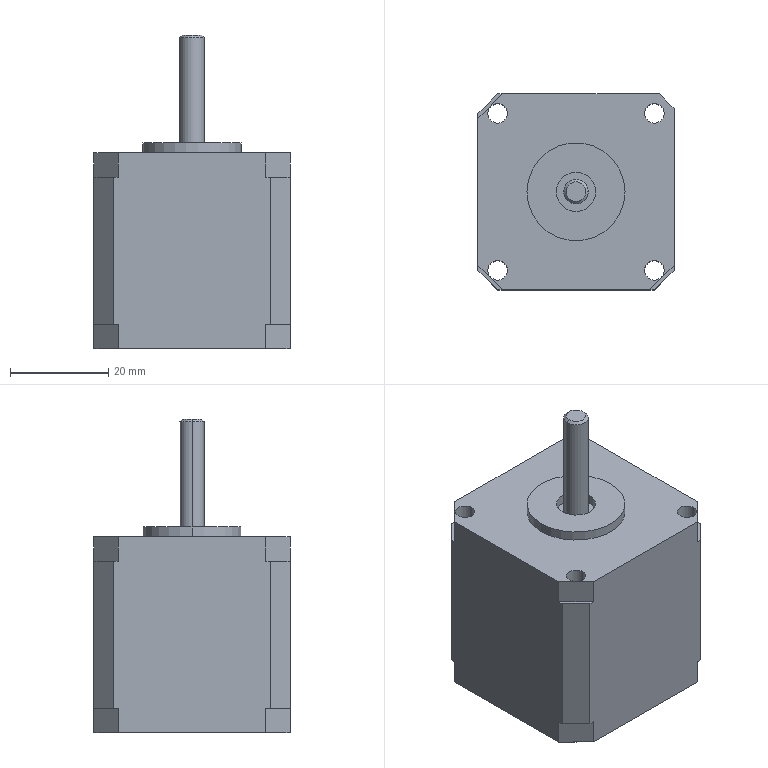Part | SolidWorks | features ICE 5, Chamfer 2, Extrusion 1, MirrorPattern 1 | 1 solid | 45 faces | box 40 x 40 x 64 mm | volume 61607 mm3 | plane 29 | cylinder 14 | cone 2 | commonest cylinder face diameters 4 x8 5 x2 8 x2 20 x2
STEP:
#1=CARTESIAN_POINT('',(-18.,16.,-20.));
#2=VERTEX_POINT('',#1);
#3=CARTESIAN_POINT('',(-14.,16.,-20.));
#4=VERTEX_POINT('',#3);
#5=CARTESIAN_POINT('',(-16.,16.,-20.));
#6=DIRECTION('',(0.,0.,1.));
#7=DIRECTION('',(1.,0.,0.));
#8=AXIS2_PLACEMENT_3D('',#5,#6,#7);
#9=CIRCLE('',#8,2.);
#10=EDGE_CURVE('',#2,#4,#9,.T.);
#11=ORIENTED_EDGE('',*,*,#10,.F.);
#12=CARTESIAN_POINT('',(-18.,16.,20.));
#13=VERTEX_POINT('',#12);
#14=CARTESIAN_POINT('',(-18.,16.,-20.));
#15=DIRECTION('',(0.,0.,1.));
#16=VECTOR('',#15,1000.);
#17=LINE('',#14,#16);
#18=EDGE_CURVE('',#2,#13,#17,.T.);
#19=ORIENTED_EDGE('',*,*,#18,.T.);
#20=CARTESIAN_POINT('',(-14.,16.,20.));
#21=VERTEX_POINT('',#20);
#22=CARTESIAN_POINT('',(-16.,16.,20.));
#23=DIRECTION('',(0.,0.,1.));
#24=DIRECTION('',(1.,0.,0.));
#25=AXIS2_PLACEMENT_3D('',#22,#23,#24);
#26=CIRCLE('',#25,2.);
#27=EDGE_CURVE('',#13,#21,#26,.T.);
#28=ORIENTED_EDGE('',*,*,#27,.T.);
#29=CARTESIAN_POINT('',(-14.,16.,-20.));
#30=DIRECTION('',(0.,0.,1.));
#31=VECTOR('',#30,1000.);
#32=LINE('',#29,#31);
#33=EDGE_CURVE('',#4,#21,#32,.T.);
#34=ORIENTED_EDGE('',*,*,#33,.F.);
#35=EDGE_LOOP('',(#11,#19,#28,#34));
#36=FACE_OUTER_BOUND('',#35,.T.);
#37=CARTESIAN_POINT('',(-16.,16.,-20.));
#38=DIRECTION('',(0.,0.,1.));
#39=DIRECTION('',(1.,0.,0.));
#40=AXIS2_PLACEMENT_3D('',#37,#38,#39);
#41=CYLINDRICAL_SURFACE('',#40,2.);
#42=ADVANCED_FACE('',(#36),#41,.F.);
#43=CARTESIAN_POINT('',(-18.,-16.,-20.));
#44=VERTEX_POINT('',#43);
#45=CARTESIAN_POINT('',(-14.,-16.,-20.));
#46=VERTEX_POINT('',#45);
#47=CARTESIAN_POINT('',(-16.,-16.,-20.));
#48=DIRECTION('',(0.,0.,1.));
#49=DIRECTION('',(1.,0.,0.));
#50=AXIS2_PLACEMENT_3D('',#47,#48,#49);
#51=CIRCLE('',#50,2.);
#52=EDGE_CURVE('',#44,#46,#51,.T.);
#53=ORIENTED_EDGE('',*,*,#52,.F.);
#54=CARTESIAN_POINT('',(-18.,-16.,20.));
#55=VERTEX_POINT('',#54);
#56=CARTESIAN_POINT('',(-18.,-16.,-20.));
#57=DIRECTION('',(0.,0.,1.));
#58=VECTOR('',#57,1000.);
#59=LINE('',#56,#58);
#60=EDGE_CURVE('',#44,#55,#59,.T.);
#61=ORIENTED_EDGE('',*,*,#60,.T.);
#62=CARTESIAN_POINT('',(-14.,-16.,20.));
#63=VERTEX_POINT('',#62);
#64=CARTESIAN_POINT('',(-16.,-16.,20.));
#65=DIRECTION('',(0.,0.,1.));
#66=DIRECTION('',(1.,0.,0.));
#67=AXIS2_PLACEMENT_3D('',#64,#65,#66);
#68=CIRCLE('',#67,2.);
#69=EDGE_CURVE('',#55,#63,#68,.T.);
#70=ORIENTED_EDGE('',*,*,#69,.T.);
#71=CARTESIAN_POINT('',(-14.,-16.,-20.));
#72=DIRECTION('',(0.,0.,1.));
#73=VECTOR('',#72,1000.);
#74=LINE('',#71,#73);
#75=EDGE_CURVE('',#46,#63,#74,.T.);
#76=ORIENTED_EDGE('',*,*,#75,.F.);
#77=EDGE_LOOP('',(#53,#61,#70,#76));
#78=FACE_OUTER_BOUND('',#77,.T.);
#79=CARTESIAN_POINT('',(-16.,-16.,-20.));
#80=DIRECTION('',(0.,0.,1.));
#81=DIRECTION('',(1.,0.,0.));
#82=AXIS2_PLACEMENT_3D('',#79,#80,#81);
#83=CYLINDRICAL_SURFACE('',#82,2.);
#84=ADVANCED_FACE('',(#78),#83,.F.);
#85=CARTESIAN_POINT('',(14.,-16.,-20.));
#86=VERTEX_POINT('',#85);
#87=CARTESIAN_POINT('',(18.,-16.,-20.));
#88=VERTEX_POINT('',#87);
#89=CARTESIAN_POINT('',(16.,-16.,-20.));
#90=DIRECTION('',(0.,0.,1.));
#91=DIRECTION('',(1.,0.,0.));
#92=AXIS2_PLACEMENT_3D('',#89,#90,#91);
#93=CIRCLE('',#92,2.);
#94=EDGE_CURVE('',#86,#88,#93,.T.);
#95=ORIENTED_EDGE('',*,*,#94,.F.);
#96=CARTESIAN_POINT('',(14.,-16.,20.));
#97=VERTEX_POINT('',#96);
#98=CARTESIAN_POINT('',(14.,-16.,-20.));
#99=DIRECTION('',(0.,0.,1.));
#100=VECTOR('',#99,1000.);
#101=LINE('',#98,#100);
#102=EDGE_CURVE('',#86,#97,#101,.T.);
#103=ORIENTED_EDGE('',*,*,#102,.T.);
#104=CARTESIAN_POINT('',(18.,-16.,20.));
#105=VERTEX_POINT('',#104);
#106=CARTESIAN_POINT('',(16.,-16.,20.));
#107=DIRECTION('',(0.,0.,1.));
#108=DIRECTION('',(1.,0.,0.));
#109=AXIS2_PLACEMENT_3D('',#106,#107,#108);
#110=CIRCLE('',#109,2.);
#111=EDGE_CURVE('',#97,#105,#110,.T.);
#112=ORIENTED_EDGE('',*,*,#111,.T.);
#113=CARTESIAN_POINT('',(18.,-16.,-20.));
#114=DIRECTION('',(0.,0.,1.));
#115=VECTOR('',#114,1000.);
#116=LINE('',#113,#115);
#117=EDGE_CURVE('',#88,#105,#116,.T.);
#118=ORIENTED_EDGE('',*,*,#117,.F.);
#119=EDGE_LOOP('',(#95,#103,#112,#118));
#120=FACE_OUTER_BOUND('',#119,.T.);
#121=CARTESIAN_POINT('',(16.,-16.,-20.));
#122=DIRECTION('',(0.,0.,1.));
#123=DIRECTION('',(1.,0.,0.));
#124=AXIS2_PLACEMENT_3D('',#121,#122,#123);
#125=CYLINDRICAL_SURFACE('',#124,2.);
#126=ADVANCED_FACE('',(#120),#125,.F.);
#127=CARTESIAN_POINT('',(14.,16.,-20.));
#128=VERTEX_POINT('',#127);
#129=CARTESIAN_POINT('',(18.,16.,-20.));
#130=VERTEX_POINT('',#129);
#131=CARTESIAN_POINT('',(16.,16.,-20.));
#132=DIRECTION('',(0.,0.,1.));
#133=DIRECTION('',(1.,0.,0.));
#134=AXIS2_PLACEMENT_3D('',#131,#132,#133);
#135=CIRCLE('',#134,2.);
#136=EDGE_CURVE('',#128,#130,#135,.T.);
#137=ORIENTED_EDGE('',*,*,#136,.F.);
#138=CARTESIAN_POINT('',(14.,16.,20.));
#139=VERTEX_POINT('',#138);
#140=CARTESIAN_POINT('',(14.,16.,-20.));
#141=DIRECTION('',(0.,0.,1.));
#142=VECTOR('',#141,1000.);
#143=LINE('',#140,#142);
#144=EDGE_CURVE('',#128,#139,#143,.T.);
#145=ORIENTED_EDGE('',*,*,#144,.T.);
#146=CARTESIAN_POINT('',(18.,16.,20.));
#147=VERTEX_POINT('',#146);
#148=CARTESIAN_POINT('',(16.,16.,20.));
#149=DIRECTION('',(0.,0.,1.));
#150=DIRECTION('',(1.,0.,0.));
#151=AXIS2_PLACEMENT_3D('',#148,#149,#150);
#152=CIRCLE('',#151,2.);
#153=EDGE_CURVE('',#139,#147,#152,.T.);
#154=ORIENTED_EDGE('',*,*,#153,.T.);
#155=CARTESIAN_POINT('',(18.,16.,-20.));
#156=DIRECTION('',(0.,0.,1.));
#157=VECTOR('',#156,1000.);
#158=LINE('',#155,#157);
#159=EDGE_CURVE('',#130,#147,#158,.T.);
#160=ORIENTED_EDGE('',*,*,#159,.F.);
#161=EDGE_LOOP('',(#137,#145,#154,#160));
#162=FACE_OUTER_BOUND('',#161,.T.);
#163=CARTESIAN_POINT('',(16.,16.,-20.));
#164=DIRECTION('',(0.,0.,1.));
#165=DIRECTION('',(1.,0.,0.));
#166=AXIS2_PLACEMENT_3D('',#163,#164,#165);
#167=CYLINDRICAL_SURFACE('',#166,2.);
#168=ADVANCED_FACE('',(#162),#167,.F.);
#169=CARTESIAN_POINT('',(2.,0.,44.));
#170=VERTEX_POINT('',#169);
#171=CARTESIAN_POINT('',(-2.,0.,44.));
#172=VERTEX_POINT('',#171);
#173=CARTESIAN_POINT('',(0.,0.,44.));
#174=DIRECTION('',(0.,0.,1.));
#175=DIRECTION('',(1.,0.,0.));
#176=AXIS2_PLACEMENT_3D('',#173,#174,#175);
#177=CIRCLE('',#176,2.);
#178=EDGE_CURVE('',#170,#172,#177,.T.);
#179=ORIENTED_EDGE('',*,*,#178,.F.);
#180=CARTESIAN_POINT('',(2.5,0.,43.5));
#181=VERTEX_POINT('',#180);
#182=CARTESIAN_POINT('',(2.,0.,44.));
#183=DIRECTION('',(0.7071,0.,-0.7071));
#184=VECTOR('',#183,1000.);
#185=LINE('',#182,#184);
#186=EDGE_CURVE('',#170,#181,#185,.T.);
#187=ORIENTED_EDGE('',*,*,#186,.T.);
#188=CARTESIAN_POINT('',(-2.5,0.,43.5));
#189=VERTEX_POINT('',#188);
#190=CARTESIAN_POINT('',(0.,0.,43.5));
#191=DIRECTION('',(0.,0.,-1.));
#192=DIRECTION('',(1.,0.,0.));
#193=AXIS2_PLACEMENT_3D('',#190,#191,#192);
#194=CIRCLE('',#193,2.5);
#195=EDGE_CURVE('',#189,#181,#194,.T.);
#196=ORIENTED_EDGE('',*,*,#195,.F.);
#197=CARTESIAN_POINT('',(-2.,0.,44.));
#198=DIRECTION('',(-0.7071,0.,-0.7071));
#199=VECTOR('',#198,1000.);
#200=LINE('',#197,#199);
#201=EDGE_CURVE('',#172,#189,#200,.T.);
#202=ORIENTED_EDGE('',*,*,#201,.F.);
#203=EDGE_LOOP('',(#179,#187,#196,#202));
#204=FACE_OUTER_BOUND('',#203,.T.);
#205=CARTESIAN_POINT('',(0.,0.,44.));
#206=DIRECTION('',(0.,0.,-1.));
#207=DIRECTION('',(-1.,0.,0.));
#208=AXIS2_PLACEMENT_3D('',#205,#206,#207);
#209=CONICAL_SURFACE('',#208,2.,0.7854);
#210=ADVANCED_FACE('',(#204),#209,.T.);
#211=ORIENTED_EDGE('',*,*,#195,.T.);
#212=CARTESIAN_POINT('',(2.5,0.,20.));
#213=VERTEX_POINT('',#212);
#214=CARTESIAN_POINT('',(2.5,0.,44.));
#215=DIRECTION('',(0.,0.,-1.));
#216=VECTOR('',#215,1000.);
#217=LINE('',#214,#216);
#218=EDGE_CURVE('',#181,#213,#217,.T.);
#219=ORIENTED_EDGE('',*,*,#218,.T.);
#220=CARTESIAN_POINT('',(-2.5,0.,20.));
#221=VERTEX_POINT('',#220);
#222=CARTESIAN_POINT('',(0.,0.,20.));
#223=DIRECTION('',(0.,0.,1.));
#224=DIRECTION('',(1.,0.,0.));
#225=AXIS2_PLACEMENT_3D('',#222,#223,#224);
#226=CIRCLE('',#225,2.5);
#227=EDGE_CURVE('',#213,#221,#226,.T.);
#228=ORIENTED_EDGE('',*,*,#227,.T.);
#229=CARTESIAN_POINT('',(-2.5,0.,44.));
#230=DIRECTION('',(0.,0.,-1.));
#231=VECTOR('',#230,1000.);
#232=LINE('',#229,#231);
#233=EDGE_CURVE('',#189,#221,#232,.T.);
#234=ORIENTED_EDGE('',*,*,#233,.F.);
#235=EDGE_LOOP('',(#211,#219,#228,#234));
#236=FACE_OUTER_BOUND('',#235,.T.);
#237=CARTESIAN_POINT('',(0.,0.,44.));
#238=DIRECTION('',(0.,0.,-1.));
#239=DIRECTION('',(-1.,0.,0.));
#240=AXIS2_PLACEMENT_3D('',#237,#238,#239);
#241=CYLINDRICAL_SURFACE('',#240,2.5);
#242=ADVANCED_FACE('',(#236),#241,.T.);
#243=CARTESIAN_POINT('',(-4.,0.,20.));
#244=VERTEX_POINT('',#243);
#245=CARTESIAN_POINT('',(4.,0.,20.));
#246=VERTEX_POINT('',#245);
#247=CARTESIAN_POINT('',(0.,0.,20.));
#248=DIRECTION('',(0.,0.,1.));
#249=DIRECTION('',(1.,0.,0.));
#250=AXIS2_PLACEMENT_3D('',#247,#248,#249);
#251=CIRCLE('',#250,4.);
#252=EDGE_CURVE('',#244,#246,#251,.T.);
#253=ORIENTED_EDGE('',*,*,#252,.F.);
#254=CARTESIAN_POINT('',(-4.,0.,22.));
#255=VERTEX_POINT('',#254);
#256=CARTESIAN_POINT('',(-4.,0.,20.));
#257=DIRECTION('',(0.,0.,1.));
#258=VECTOR('',#257,1000.);
#259=LINE('',#256,#258);
#260=EDGE_CURVE('',#244,#255,#259,.T.);
#261=ORIENTED_EDGE('',*,*,#260,.T.);
#262=CARTESIAN_POINT('',(4.,0.,22.));
#263=VERTEX_POINT('',#262);
#264=CARTESIAN_POINT('',(0.,0.,22.));
#265=DIRECTION('',(0.,0.,1.));
#266=DIRECTION('',(1.,0.,0.));
#267=AXIS2_PLACEMENT_3D('',#264,#265,#266);
#268=CIRCLE('',#267,4.);
#269=EDGE_CURVE('',#255,#263,#268,.T.);
#270=ORIENTED_EDGE('',*,*,#269,.T.);
#271=CARTESIAN_POINT('',(4.,0.,20.));
#272=DIRECTION('',(0.,0.,1.));
#273=VECTOR('',#272,1000.);
#274=LINE('',#271,#273);
#275=EDGE_CURVE('',#246,#263,#274,.T.);
#276=ORIENTED_EDGE('',*,*,#275,.F.);
#277=EDGE_LOOP('',(#253,#261,#270,#276));
#278=FACE_OUTER_BOUND('',#277,.T.);
#279=CARTESIAN_POINT('',(0.,0.,20.));
#280=DIRECTION('',(0.,0.,1.));
#281=DIRECTION('',(1.,0.,0.));
#282=AXIS2_PLACEMENT_3D('',#279,#280,#281);
#283=CYLINDRICAL_SURFACE('',#282,4.);
#284=ADVANCED_FACE('',(#278),#283,.F.);
#285=CARTESIAN_POINT('',(10.,0.,22.));
#286=VERTEX_POINT('',#285);
#287=CARTESIAN_POINT('',(-10.,0.,22.));
#288=VERTEX_POINT('',#287);
#289=CARTESIAN_POINT('',(0.,0.,22.));
#290=DIRECTION('',(0.,0.,1.));
#291=DIRECTION('',(1.,0.,0.));
#292=AXIS2_PLACEMENT_3D('',#289,#290,#291);
#293=CIRCLE('',#292,10.);
#294=EDGE_CURVE('',#286,#288,#293,.T.);
#295=ORIENTED_EDGE('',*,*,#294,.F.);
#296=CARTESIAN_POINT('',(10.,0.,20.));
#297=VERTEX_POINT('',#296);
#298=CARTESIAN_POINT('',(10.,0.,22.));
#299=DIRECTION('',(0.,0.,-1.));
#300=VECTOR('',#299,1000.);
#301=LINE('',#298,#300);
#302=EDGE_CURVE('',#286,#297,#301,.T.);
#303=ORIENTED_EDGE('',*,*,#302,.T.);
#304=CARTESIAN_POINT('',(-10.,0.,20.));
#305=VERTEX_POINT('',#304);
#306=CARTESIAN_POINT('',(0.,0.,20.));
#307=DIRECTION('',(0.,0.,1.));
#308=DIRECTION('',(-1.,0.,0.));
#309=AXIS2_PLACEMENT_3D('',#306,#307,#308);
#310=CIRCLE('',#309,10.);
#311=EDGE_CURVE('',#297,#305,#310,.T.);
#312=ORIENTED_EDGE('',*,*,#311,.T.);
#313=CARTESIAN_POINT('',(-10.,0.,22.));
#314=DIRECTION('',(0.,0.,-1.));
#315=VECTOR('',#314,1000.);
#316=LINE('',#313,#315);
#317=EDGE_CURVE('',#288,#305,#316,.T.);
#318=ORIENTED_EDGE('',*,*,#317,.F.);
#319=EDGE_LOOP('',(#295,#303,#312,#318));
#320=FACE_OUTER_BOUND('',#319,.T.);
#321=CARTESIAN_POINT('',(0.,0.,22.));
#322=DIRECTION('',(0.,0.,-1.));
#323=DIRECTION('',(-1.,0.,0.));
#324=AXIS2_PLACEMENT_3D('',#321,#322,#323);
#325=CYLINDRICAL_SURFACE('',#324,10.);
#326=ADVANCED_FACE('',(#320),#325,.T.);
#327=CARTESIAN_POINT('',(0.,0.,22.));
#328=DIRECTION('',(0.,0.,1.));
#329=DIRECTION('',(1.,0.,0.));
#330=AXIS2_PLACEMENT_3D('',#327,#328,#329);
#331=CIRCLE('',#330,4.);
#332=EDGE_CURVE('',#263,#255,#331,.T.);
#333=ORIENTED_EDGE('',*,*,#332,.F.);
#334=ORIENTED_EDGE('',*,*,#269,.F.);
#335=EDGE_LOOP('',(#333,#334));
#336=FACE_BOUND('',#335,.T.);
#337=CARTESIAN_POINT('',(0.,0.,22.));
#338=DIRECTION('',(0.,0.,1.));
#339=DIRECTION('',(1.,0.,0.));
#340=AXIS2_PLACEMENT_3D('',#337,#338,#339);
#341=CIRCLE('',#340,10.);
#342=EDGE_CURVE('',#288,#286,#341,.T.);
#343=ORIENTED_EDGE('',*,*,#342,.T.);
#344=ORIENTED_EDGE('',*,*,#294,.T.);
#345=EDGE_LOOP('',(#343,#344));
#346=FACE_OUTER_BOUND('',#345,.T.);
#347=CARTESIAN_POINT('',(0.,0.,22.));
#348=DIRECTION('',(0.,0.,1.));
#349=DIRECTION('',(1.,0.,0.));
#350=AXIS2_PLACEMENT_3D('',#347,#348,#349);
#351=PLANE('',#350);
#352=ADVANCED_FACE('',(#336,#346),#351,.T.);
#353=CARTESIAN_POINT('',(-16.,16.,20.));
#354=DIRECTION('',(0.,0.,1.));
#355=DIRECTION('',(1.,0.,0.));
#356=AXIS2_PLACEMENT_3D('',#353,#354,#355);
#357=CIRCLE('',#356,2.);
#358=EDGE_CURVE('',#21,#13,#357,.T.);
#359=ORIENTED_EDGE('',*,*,#358,.F.);
#360=ORIENTED_EDGE('',*,*,#27,.F.);
#361=EDGE_LOOP('',(#359,#360));
#362=FACE_BOUND('',#361,.T.);
#363=CARTESIAN_POINT('',(-16.,-16.,20.));
#364=DIRECTION('',(0.,0.,1.));
#365=DIRECTION('',(1.,0.,0.));
#366=AXIS2_PLACEMENT_3D('',#363,#364,#365);
#367=CIRCLE('',#366,2.);
#368=EDGE_CURVE('',#63,#55,#367,.T.);
#369=ORIENTED_EDGE('',*,*,#368,.F.);
#370=ORIENTED_EDGE('',*,*,#69,.F.);
#371=EDGE_LOOP('',(#369,#370));
#372=FACE_BOUND('',#371,.T.);
#373=CARTESIAN_POINT('',(16.,-16.,20.));
#374=DIRECTION('',(0.,0.,1.));
#375=DIRECTION('',(1.,0.,0.));
#376=AXIS2_PLACEMENT_3D('',#373,#374,#375);
#377=CIRCLE('',#376,2.);
#378=EDGE_CURVE('',#105,#97,#377,.T.);
#379=ORIENTED_EDGE('',*,*,#378,.F.);
#380=ORIENTED_EDGE('',*,*,#111,.F.);
#381=EDGE_LOOP('',(#379,#380));
#382=FACE_BOUND('',#381,.T.);
#383=CARTESIAN_POINT('',(16.,16.,20.));
#384=DIRECTION('',(0.,0.,1.));
#385=DIRECTION('',(1.,0.,0.));
#386=AXIS2_PLACEMENT_3D('',#383,#384,#385);
#387=CIRCLE('',#386,2.);
#388=EDGE_CURVE('',#147,#139,#387,.T.);
#389=ORIENTED_EDGE('',*,*,#388,.F.);
#390=ORIENTED_EDGE('',*,*,#153,.F.);
#391=EDGE_LOOP('',(#389,#390));
#392=FACE_BOUND('',#391,.T.);
#393=CARTESIAN_POINT('',(-15.,20.,20.));
#394=VERTEX_POINT('',#393);
#395=CARTESIAN_POINT('',(-20.,15.,20.));
#396=VERTEX_POINT('',#395);
#397=CARTESIAN_POINT('',(-15.,20.,20.));
#398=DIRECTION('',(-0.7071,-0.7071,0.));
#399=VECTOR('',#398,1000.);
#400=LINE('',#397,#399);
#401=EDGE_CURVE('',#394,#396,#400,.T.);
#402=ORIENTED_EDGE('',*,*,#401,.T.);
#403=CARTESIAN_POINT('',(-20.,-15.,20.));
#404=VERTEX_POINT('',#403);
#405=CARTESIAN_POINT('',(-20.,-15.,20.));
#406=DIRECTION('',(0.,-1.,0.));
#407=VECTOR('',#406,1000.);
#408=LINE('',#405,#407);
#409=EDGE_CURVE('',#396,#404,#408,.T.);
#410=ORIENTED_EDGE('',*,*,#409,.T.);
#411=CARTESIAN_POINT('',(-15.,-20.,20.));
#412=VERTEX_POINT('',#411);
#413=CARTESIAN_POINT('',(-15.,-20.,20.));
#414=DIRECTION('',(0.7071,-0.7071,0.));
#415=VECTOR('',#414,1000.);
#416=LINE('',#413,#415);
#417=EDGE_CURVE('',#404,#412,#416,.T.);
#418=ORIENTED_EDGE('',*,*,#417,.T.);
#419=CARTESIAN_POINT('',(15.,-20.,20.));
#420=VERTEX_POINT('',#419);
#421=CARTESIAN_POINT('',(15.,-20.,20.));
#422=DIRECTION('',(1.,0.,0.));
#423=VECTOR('',#422,1000.);
#424=LINE('',#421,#423);
#425=EDGE_CURVE('',#412,#420,#424,.T.);
#426=ORIENTED_EDGE('',*,*,#425,.T.);
#427=CARTESIAN_POINT('',(20.,-15.,20.));
#428=VERTEX_POINT('',#427);
#429=CARTESIAN_POINT('',(20.,-15.,20.));
#430=DIRECTION('',(0.7071,0.7071,0.));
#431=VECTOR('',#430,1000.);
#432=LINE('',#429,#431);
#433=EDGE_CURVE('',#420,#428,#432,.T.);
#434=ORIENTED_EDGE('',*,*,#433,.T.);
#435=CARTESIAN_POINT('',(20.,17.,20.));
#436=VERTEX_POINT('',#435);
#437=CARTESIAN_POINT('',(20.,-15.,20.));
#438=DIRECTION('',(0.,1.,0.));
#439=VECTOR('',#438,1000.);
#440=LINE('',#437,#439);
#441=EDGE_CURVE('',#428,#436,#440,.T.);
#442=ORIENTED_EDGE('',*,*,#441,.T.);
#443=CARTESIAN_POINT('',(17.,20.,20.));
#444=VERTEX_POINT('',#443);
#445=CARTESIAN_POINT('',(20.,17.,20.));
#446=DIRECTION('',(-0.7071,0.7071,0.));
#447=VECTOR('',#446,1000.);
#448=LINE('',#445,#447);
#449=EDGE_CURVE('',#436,#444,#448,.T.);
#450=ORIENTED_EDGE('',*,*,#449,.T.);
#451=CARTESIAN_POINT('',(17.,20.,20.));
#452=DIRECTION('',(-1.,0.,0.));
#453=VECTOR('',#452,1000.);
#454=LINE('',#451,#453);
#455=EDGE_CURVE('',#444,#394,#454,.T.);
#456=ORIENTED_EDGE('',*,*,#455,.T.);
#457=EDGE_LOOP('',(#402,#410,#418,#426,#434,#442,#450,#456));
#458=FACE_OUTER_BOUND('',#457,.T.);
#459=CARTESIAN_POINT('',(0.,0.,20.));
#460=DIRECTION('',(0.,0.,1.));
#461=DIRECTION('',(-1.,0.,0.));
#462=AXIS2_PLACEMENT_3D('',#459,#460,#461);
#463=CIRCLE('',#462,10.);
#464=EDGE_CURVE('',#305,#297,#463,.T.);
#465=ORIENTED_EDGE('',*,*,#464,.F.);
#466=ORIENTED_EDGE('',*,*,#311,.F.);
#467=EDGE_LOOP('',(#465,#466));
#468=FACE_BOUND('',#467,.T.);
#469=CARTESIAN_POINT('',(0.,0.,20.));
#470=DIRECTION('',(0.,0.,-1.));
#471=DIRECTION('',(-1.,0.,0.));
#472=AXIS2_PLACEMENT_3D('',#469,#470,#471);
#473=PLANE('',#472);
#474=ADVANCED_FACE('',(#362,#372,#382,#392,#458,#468),#473,.F.);
#475=CARTESIAN_POINT('',(-15.,20.,-15.));
#476=VERTEX_POINT('',#475);
#477=CARTESIAN_POINT('',(-16.,20.,-15.));
#478=VERTEX_POINT('',#477);
#479=CARTESIAN_POINT('',(20.,20.,-15.));
#480=DIRECTION('',(-1.,0.,0.));
#481=VECTOR('',#480,1000.);
#482=LINE('',#479,#481);
#483=EDGE_CURVE('',#476,#478,#482,.T.);
#484=ORIENTED_EDGE('',*,*,#483,.F.);
#485=CARTESIAN_POINT('',(-20.,15.,-15.));
#486=VERTEX_POINT('',#485);
#487=CARTESIAN_POINT('',(-15.,20.,-15.));
#488=DIRECTION('',(-0.7071,-0.7071,0.));
#489=VECTOR('',#488,1000.);
#490=LINE('',#487,#489);
#491=EDGE_CURVE('',#476,#486,#490,.T.);
#492=ORIENTED_EDGE('',*,*,#491,.T.);
#493=CARTESIAN_POINT('',(-20.,16.,-15.));
#494=VERTEX_POINT('',#493);
#495=CARTESIAN_POINT('',(-20.,-20.,-15.));
#496=DIRECTION('',(0.,-1.,0.));
#497=VECTOR('',#496,1000.);
#498=LINE('',#495,#497);
#499=EDGE_CURVE('',#494,#486,#498,.T.);
#500=ORIENTED_EDGE('',*,*,#499,.F.);
#501=CARTESIAN_POINT('',(-20.,16.,-15.));
#502=DIRECTION('',(0.7071,0.7071,0.));
#503=VECTOR('',#502,1000.);
#504=LINE('',#501,#503);
#505=EDGE_CURVE('',#494,#478,#504,.T.);
#506=ORIENTED_EDGE('',*,*,#505,.T.);
#507=EDGE_LOOP('',(#484,#492,#500,#506));
#508=FACE_OUTER_BOUND('',#507,.T.);
#509=CARTESIAN_POINT('',(0.,0.,-15.));
#510=DIRECTION('',(0.,0.,1.));
#511=DIRECTION('',(1.,0.,0.));
#512=AXIS2_PLACEMENT_3D('',#509,#510,#511);
#513=PLANE('',#512);
#514=ADVANCED_FACE('',(#508),#513,.F.);
#515=CARTESIAN_POINT('',(-20.,-15.,-15.));
#516=VERTEX_POINT('',#515);
#517=CARTESIAN_POINT('',(-20.,-16.,-15.));
#518=VERTEX_POINT('',#517);
#519=CARTESIAN_POINT('',(-20.,-20.,-15.));
#520=DIRECTION('',(0.,-1.,0.));
#521=VECTOR('',#520,1000.);
#522=LINE('',#519,#521);
#523=EDGE_CURVE('',#516,#518,#522,.T.);
#524=ORIENTED_EDGE('',*,*,#523,.F.);
#525=CARTESIAN_POINT('',(-15.,-20.,-15.));
#526=VERTEX_POINT('',#525);
#527=CARTESIAN_POINT('',(-15.,-20.,-15.));
#528=DIRECTION('',(0.7071,-0.7071,0.));
#529=VECTOR('',#528,1000.);
#530=LINE('',#527,#529);
#531=EDGE_CURVE('',#516,#526,#530,.T.);
#532=ORIENTED_EDGE('',*,*,#531,.T.);
#533=CARTESIAN_POINT('',(-16.,-20.,-15.));
#534=VERTEX_POINT('',#533);
#535=CARTESIAN_POINT('',(20.,-20.,-15.));
#536=DIRECTION('',(1.,0.,0.));
#537=VECTOR('',#536,1000.);
#538=LINE('',#535,#537);
#539=EDGE_CURVE('',#534,#526,#538,.T.);
#540=ORIENTED_EDGE('',*,*,#539,.F.);
#541=CARTESIAN_POINT('',(-16.,-20.,-15.));
#542=DIRECTION('',(-0.7071,0.7071,0.));
#543=VECTOR('',#542,1000.);
#544=LINE('',#541,#543);
#545=EDGE_CURVE('',#534,#518,#544,.T.);
#546=ORIENTED_EDGE('',*,*,#545,.T.);
#547=EDGE_LOOP('',(#524,#532,#540,#546));
#548=FACE_OUTER_BOUND('',#547,.T.);
#549=CARTESIAN_POINT('',(0.,0.,-15.));
#550=DIRECTION('',(0.,0.,1.));
#551=DIRECTION('',(1.,0.,0.));
#552=AXIS2_PLACEMENT_3D('',#549,#550,#551);
#553=PLANE('',#552);
#554=ADVANCED_FACE('',(#548),#553,.F.);
#555=CARTESIAN_POINT('',(-15.,20.,15.));
#556=VERTEX_POINT('',#555);
#557=CARTESIAN_POINT('',(-20.,15.,15.));
#558=VERTEX_POINT('',#557);
#559=CARTESIAN_POINT('',(-15.,20.,15.));
#560=DIRECTION('',(-0.7071,-0.7071,0.));
#561=VECTOR('',#560,1000.);
#562=LINE('',#559,#561);
#563=EDGE_CURVE('',#556,#558,#562,.T.);
#564=ORIENTED_EDGE('',*,*,#563,.F.);
#565=CARTESIAN_POINT('',(-16.,20.,15.));
#566=VERTEX_POINT('',#565);
#567=CARTESIAN_POINT('',(20.,20.,15.));
#568=DIRECTION('',(-1.,0.,0.));
#569=VECTOR('',#568,1000.);
#570=LINE('',#567,#569);
#571=EDGE_CURVE('',#556,#566,#570,.T.);
#572=ORIENTED_EDGE('',*,*,#571,.T.);
#573=CARTESIAN_POINT('',(-20.,16.,15.));
#574=VERTEX_POINT('',#573);
#575=CARTESIAN_POINT('',(-18.,18.,15.));
#576=DIRECTION('',(-0.7071,-0.7071,0.));
#577=VECTOR('',#576,1000.);
#578=LINE('',#575,#577);
#579=EDGE_CURVE('',#566,#574,#578,.T.);
#580=ORIENTED_EDGE('',*,*,#579,.T.);
#581=CARTESIAN_POINT('',(-20.,-20.,15.));
#582=DIRECTION('',(0.,-1.,0.));
#583=VECTOR('',#582,1000.);
#584=LINE('',#581,#583);
#585=EDGE_CURVE('',#574,#558,#584,.T.);
#586=ORIENTED_EDGE('',*,*,#585,.T.);
#587=EDGE_LOOP('',(#564,#572,#580,#586));
#588=FACE_OUTER_BOUND('',#587,.T.);
#589=CARTESIAN_POINT('',(0.,0.,15.));
#590=DIRECTION('',(0.,0.,1.));
#591=DIRECTION('',(1.,0.,0.));
#592=AXIS2_PLACEMENT_3D('',#589,#590,#591);
#593=PLANE('',#592);
#594=ADVANCED_FACE('',(#588),#593,.T.);
#595=CARTESIAN_POINT('',(15.,-20.,15.));
#596=VERTEX_POINT('',#595);
#597=CARTESIAN_POINT('',(20.,-15.,15.));
#598=VERTEX_POINT('',#597);
#599=CARTESIAN_POINT('',(20.,-15.,15.));
#600=DIRECTION('',(0.7071,0.7071,0.));
#601=VECTOR('',#600,1000.);
#602=LINE('',#599,#601);
#603=EDGE_CURVE('',#596,#598,#602,.T.);
#604=ORIENTED_EDGE('',*,*,#603,.F.);
#605=CARTESIAN_POINT('',(16.,-20.,15.));
#606=VERTEX_POINT('',#605);
#607=CARTESIAN_POINT('',(20.,-20.,15.));
#608=DIRECTION('',(1.,0.,0.));
#609=VECTOR('',#608,1000.);
#610=LINE('',#607,#609);
#611=EDGE_CURVE('',#596,#606,#610,.T.);
#612=ORIENTED_EDGE('',*,*,#611,.T.);
#613=CARTESIAN_POINT('',(20.,-16.,15.));
#614=VERTEX_POINT('',#613);
#615=CARTESIAN_POINT('',(18.,-18.,15.));
#616=DIRECTION('',(0.7071,0.7071,0.));
#617=VECTOR('',#616,1000.);
#618=LINE('',#615,#617);
#619=EDGE_CURVE('',#606,#614,#618,.T.);
#620=ORIENTED_EDGE('',*,*,#619,.T.);
#621=CARTESIAN_POINT('',(20.,-20.,15.));
#622=DIRECTION('',(0.,1.,0.));
#623=VECTOR('',#622,1000.);
#624=LINE('',#621,#623);
#625=EDGE_CURVE('',#614,#598,#624,.T.);
#626=ORIENTED_EDGE('',*,*,#625,.T.);
#627=EDGE_LOOP('',(#604,#612,#620,#626));
#628=FACE_OUTER_BOUND('',#627,.T.);
#629=CARTESIAN_POINT('',(0.,0.,15.));
#630=DIRECTION('',(0.,0.,1.));
#631=DIRECTION('',(1.,0.,0.));
#632=AXIS2_PLACEMENT_3D('',#629,#630,#631);
#633=PLANE('',#632);
#634=ADVANCED_FACE('',(#628),#633,.T.);
#635=ORIENTED_EDGE('',*,*,#499,.T.);
#636=CARTESIAN_POINT('',(-20.,15.,-20.));
#637=VERTEX_POINT('',#636);
#638=CARTESIAN_POINT('',(-20.,15.,-20.));
#639=DIRECTION('',(0.,0.,1.));
#640=VECTOR('',#639,1000.);
#641=LINE('',#638,#640);
#642=EDGE_CURVE('',#637,#486,#641,.T.);
#643=ORIENTED_EDGE('',*,*,#642,.F.);
#644=CARTESIAN_POINT('',(-20.,-15.,-20.));
#645=VERTEX_POINT('',#644);
#646=CARTESIAN_POINT('',(-20.,-15.,-20.));
#647=DIRECTION('',(0.,-1.,0.));
#648=VECTOR('',#647,1000.);
#649=LINE('',#646,#648);
#650=EDGE_CURVE('',#637,#645,#649,.T.);
#651=ORIENTED_EDGE('',*,*,#650,.T.);
#652=CARTESIAN_POINT('',(-20.,-15.,-20.));
#653=DIRECTION('',(0.,0.,1.));
#654=VECTOR('',#653,1000.);
#655=LINE('',#652,#654);
#656=EDGE_CURVE('',#645,#516,#655,.T.);
#657=ORIENTED_EDGE('',*,*,#656,.T.);
#658=ORIENTED_EDGE('',*,*,#523,.T.);
#659=CARTESIAN_POINT('',(-20.,-16.,15.));
#660=VERTEX_POINT('',#659);
#661=CARTESIAN_POINT('',(-20.,-16.,15.));
#662=DIRECTION('',(0.,0.,1.));
#663=VECTOR('',#662,1000.);
#664=LINE('',#661,#663);
#665=EDGE_CURVE('',#518,#660,#664,.T.);
#666=ORIENTED_EDGE('',*,*,#665,.T.);
#667=CARTESIAN_POINT('',(-20.,-15.,15.));
#668=VERTEX_POINT('',#667);
#669=CARTESIAN_POINT('',(-20.,-20.,15.));
#670=DIRECTION('',(0.,-1.,0.));
#671=VECTOR('',#670,1000.);
#672=LINE('',#669,#671);
#673=EDGE_CURVE('',#668,#660,#672,.T.);
#674=ORIENTED_EDGE('',*,*,#673,.F.);
#675=CARTESIAN_POINT('',(-20.,-15.,20.));
#676=DIRECTION('',(0.,0.,-1.));
#677=VECTOR('',#676,1000.);
#678=LINE('',#675,#677);
#679=EDGE_CURVE('',#404,#668,#678,.T.);
#680=ORIENTED_EDGE('',*,*,#679,.F.);
#681=ORIENTED_EDGE('',*,*,#409,.F.);
#682=CARTESIAN_POINT('',(-20.,15.,20.));
#683=DIRECTION('',(0.,0.,-1.));
#684=VECTOR('',#683,1000.);
#685=LINE('',#682,#684);
#686=EDGE_CURVE('',#396,#558,#685,.T.);
#687=ORIENTED_EDGE('',*,*,#686,.T.);
#688=ORIENTED_EDGE('',*,*,#585,.F.);
#689=CARTESIAN_POINT('',(-20.,16.,15.));
#690=DIRECTION('',(0.,0.,-1.));
#691=VECTOR('',#690,1000.);
#692=LINE('',#689,#691);
#693=EDGE_CURVE('',#574,#494,#692,.T.);
#694=ORIENTED_EDGE('',*,*,#693,.T.);
#695=EDGE_LOOP('',(#635,#643,#651,#657,#658,#666,#674,#680,#681,#687,#688,#694));
#696=FACE_OUTER_BOUND('',#695,.T.);
#697=CARTESIAN_POINT('',(-20.,-20.,15.));
#698=DIRECTION('',(1.,0.,0.));
#699=DIRECTION('',(0.,0.,-1.));
#700=AXIS2_PLACEMENT_3D('',#697,#698,#699);
#701=PLANE('',#700);
#702=ADVANCED_FACE('',(#696),#701,.F.);
#703=CARTESIAN_POINT('',(-16.,-20.,15.));
#704=VERTEX_POINT('',#703);
#705=CARTESIAN_POINT('',(-15.,-20.,15.));
#706=VERTEX_POINT('',#705);
#707=CARTESIAN_POINT('',(20.,-20.,15.));
#708=DIRECTION('',(1.,0.,0.));
#709=VECTOR('',#708,1000.);
#710=LINE('',#707,#709);
#711=EDGE_CURVE('',#704,#706,#710,.T.);
#712=ORIENTED_EDGE('',*,*,#711,.F.);
#713=CARTESIAN_POINT('',(-16.,-20.,15.));
#714=DIRECTION('',(0.,0.,-1.));
#715=VECTOR('',#714,1000.);
#716=LINE('',#713,#715);
#717=EDGE_CURVE('',#704,#534,#716,.T.);
#718=ORIENTED_EDGE('',*,*,#717,.T.);
#719=ORIENTED_EDGE('',*,*,#539,.T.);
#720=CARTESIAN_POINT('',(-15.,-20.,-20.));
#721=VERTEX_POINT('',#720);
#722=CARTESIAN_POINT('',(-15.,-20.,-20.));
#723=DIRECTION('',(0.,0.,1.));
#724=VECTOR('',#723,1000.);
#725=LINE('',#722,#724);
#726=EDGE_CURVE('',#721,#526,#725,.T.);
#727=ORIENTED_EDGE('',*,*,#726,.F.);
#728=CARTESIAN_POINT('',(15.,-20.,-20.));
#729=VERTEX_POINT('',#728);
#730=CARTESIAN_POINT('',(15.,-20.,-20.));
#731=DIRECTION('',(1.,0.,0.));
#732=VECTOR('',#731,1000.);
#733=LINE('',#730,#732);
#734=EDGE_CURVE('',#721,#729,#733,.T.);
#735=ORIENTED_EDGE('',*,*,#734,.T.);
#736=CARTESIAN_POINT('',(15.,-20.,-15.));
#737=VERTEX_POINT('',#736);
#738=CARTESIAN_POINT('',(15.,-20.,-20.));
#739=DIRECTION('',(0.,0.,1.));
#740=VECTOR('',#739,1000.);
#741=LINE('',#738,#740);
#742=EDGE_CURVE('',#729,#737,#741,.T.);
#743=ORIENTED_EDGE('',*,*,#742,.T.);
#744=CARTESIAN_POINT('',(16.,-20.,-15.));
#745=VERTEX_POINT('',#744);
#746=CARTESIAN_POINT('',(20.,-20.,-15.));
#747=DIRECTION('',(1.,0.,0.));
#748=VECTOR('',#747,1000.);
#749=LINE('',#746,#748);
#750=EDGE_CURVE('',#737,#745,#749,.T.);
#751=ORIENTED_EDGE('',*,*,#750,.T.);
#752=CARTESIAN_POINT('',(16.,-20.,15.));
#753=DIRECTION('',(0.,0.,1.));
#754=VECTOR('',#753,1000.);
#755=LINE('',#752,#754);
#756=EDGE_CURVE('',#745,#606,#755,.T.);
#757=ORIENTED_EDGE('',*,*,#756,.T.);
#758=ORIENTED_EDGE('',*,*,#611,.F.);
#759=CARTESIAN_POINT('',(15.,-20.,20.));
#760=DIRECTION('',(0.,0.,-1.));
#761=VECTOR('',#760,1000.);
#762=LINE('',#759,#761);
#763=EDGE_CURVE('',#420,#596,#762,.T.);
#764=ORIENTED_EDGE('',*,*,#763,.F.);
#765=ORIENTED_EDGE('',*,*,#425,.F.);
#766=CARTESIAN_POINT('',(-15.,-20.,20.));
#767=DIRECTION('',(0.,0.,-1.));
#768=VECTOR('',#767,1000.);
#769=LINE('',#766,#768);
#770=EDGE_CURVE('',#412,#706,#769,.T.);
#771=ORIENTED_EDGE('',*,*,#770,.T.);
#772=EDGE_LOOP('',(#712,#718,#719,#727,#735,#743,#751,#757,#758,#764,#765,#771));
#773=FACE_OUTER_BOUND('',#772,.T.);
#774=CARTESIAN_POINT('',(20.,-20.,15.));
#775=DIRECTION('',(0.,1.,0.));
#776=DIRECTION('',(-1.,0.,0.));
#777=AXIS2_PLACEMENT_3D('',#774,#775,#776);
#778=PLANE('',#777);
#779=ADVANCED_FACE('',(#773),#778,.F.);
#780=ORIENTED_EDGE('',*,*,#625,.F.);
#781=CARTESIAN_POINT('',(20.,-16.,-15.));
#782=VERTEX_POINT('',#781);
#783=CARTESIAN_POINT('',(20.,-16.,15.));
#784=DIRECTION('',(0.,0.,-1.));
#785=VECTOR('',#784,1000.);
#786=LINE('',#783,#785);
#787=EDGE_CURVE('',#614,#782,#786,.T.);
#788=ORIENTED_EDGE('',*,*,#787,.T.);
#789=CARTESIAN_POINT('',(20.,-15.,-15.));
#790=VERTEX_POINT('',#789);
#791=CARTESIAN_POINT('',(20.,-20.,-15.));
#792=DIRECTION('',(0.,1.,0.));
#793=VECTOR('',#792,1000.);
#794=LINE('',#791,#793);
#795=EDGE_CURVE('',#782,#790,#794,.T.);
#796=ORIENTED_EDGE('',*,*,#795,.T.);
#797=CARTESIAN_POINT('',(20.,-15.,-20.));
#798=VERTEX_POINT('',#797);
#799=CARTESIAN_POINT('',(20.,-15.,-20.));
#800=DIRECTION('',(0.,0.,1.));
#801=VECTOR('',#800,1000.);
#802=LINE('',#799,#801);
#803=EDGE_CURVE('',#798,#790,#802,.T.);
#804=ORIENTED_EDGE('',*,*,#803,.F.);
#805=CARTESIAN_POINT('',(20.,17.,-20.));
#806=VERTEX_POINT('',#805);
#807=CARTESIAN_POINT('',(20.,-15.,-20.));
#808=DIRECTION('',(0.,1.,0.));
#809=VECTOR('',#808,1000.);
#810=LINE('',#807,#809);
#811=EDGE_CURVE('',#798,#806,#810,.T.);
#812=ORIENTED_EDGE('',*,*,#811,.T.);
#813=CARTESIAN_POINT('',(20.,17.,-15.));
#814=VERTEX_POINT('',#813);
#815=CARTESIAN_POINT('',(20.,17.,-20.));
#816=DIRECTION('',(0.,0.,1.));
#817=VECTOR('',#816,1000.);
#818=LINE('',#815,#817);
#819=EDGE_CURVE('',#806,#814,#818,.T.);
#820=ORIENTED_EDGE('',*,*,#819,.T.);
#821=CARTESIAN_POINT('',(20.,16.,-15.));
#822=VERTEX_POINT('',#821);
#823=CARTESIAN_POINT('',(20.,-15.,-15.));
#824=DIRECTION('',(0.,1.,0.));
#825=VECTOR('',#824,1000.);
#826=LINE('',#823,#825);
#827=EDGE_CURVE('',#822,#814,#826,.T.);
#828=ORIENTED_EDGE('',*,*,#827,.F.);
#829=CARTESIAN_POINT('',(20.,16.,15.));
#830=VERTEX_POINT('',#829);
#831=CARTESIAN_POINT('',(20.,16.,15.));
#832=DIRECTION('',(0.,0.,1.));
#833=VECTOR('',#832,1000.);
#834=LINE('',#831,#833);
#835=EDGE_CURVE('',#822,#830,#834,.T.);
#836=ORIENTED_EDGE('',*,*,#835,.T.);
#837=CARTESIAN_POINT('',(20.,17.,15.));
#838=VERTEX_POINT('',#837);
#839=CARTESIAN_POINT('',(20.,-15.,15.));
#840=DIRECTION('',(0.,1.,0.));
#841=VECTOR('',#840,1000.);
#842=LINE('',#839,#841);
#843=EDGE_CURVE('',#830,#838,#842,.T.);
#844=ORIENTED_EDGE('',*,*,#843,.T.);
#845=CARTESIAN_POINT('',(20.,17.,20.));
#846=DIRECTION('',(0.,0.,-1.));
#847=VECTOR('',#846,1000.);
#848=LINE('',#845,#847);
#849=EDGE_CURVE('',#436,#838,#848,.T.);
#850=ORIENTED_EDGE('',*,*,#849,.F.);
#851=ORIENTED_EDGE('',*,*,#441,.F.);
#852=CARTESIAN_POINT('',(20.,-15.,20.));
#853=DIRECTION('',(0.,0.,-1.));
#854=VECTOR('',#853,1000.);
#855=LINE('',#852,#854);
#856=EDGE_CURVE('',#428,#598,#855,.T.);
#857=ORIENTED_EDGE('',*,*,#856,.T.);
#858=EDGE_LOOP('',(#780,#788,#796,#804,#812,#820,#828,#836,#844,#850,#851,#857));
#859=FACE_OUTER_BOUND('',#858,.T.);
#860=CARTESIAN_POINT('',(20.,-20.,15.));
#861=DIRECTION('',(-1.,0.,0.));
#862=DIRECTION('',(0.,0.,1.));
#863=AXIS2_PLACEMENT_3D('',#860,#861,#862);
#864=PLANE('',#863);
#865=ADVANCED_FACE('',(#859),#864,.F.);
#866=CARTESIAN_POINT('',(16.,20.,15.));
#867=VERTEX_POINT('',#866);
#868=CARTESIAN_POINT('',(16.,20.,-15.));
#869=VERTEX_POINT('',#868);
#870=CARTESIAN_POINT('',(16.,20.,15.));
#871=DIRECTION('',(0.,0.,-1.));
#872=VECTOR('',#871,1000.);
#873=LINE('',#870,#872);
#874=EDGE_CURVE('',#867,#869,#873,.T.);
#875=ORIENTED_EDGE('',*,*,#874,.T.);
#876=CARTESIAN_POINT('',(17.,20.,-15.));
#877=VERTEX_POINT('',#876);
#878=CARTESIAN_POINT('',(17.,20.,-15.));
#879=DIRECTION('',(-1.,0.,0.));
#880=VECTOR('',#879,1000.);
#881=LINE('',#878,#880);
#882=EDGE_CURVE('',#877,#869,#881,.T.);
#883=ORIENTED_EDGE('',*,*,#882,.F.);
#884=CARTESIAN_POINT('',(17.,20.,-20.));
#885=VERTEX_POINT('',#884);
#886=CARTESIAN_POINT('',(17.,20.,-20.));
#887=DIRECTION('',(0.,0.,1.));
#888=VECTOR('',#887,1000.);
#889=LINE('',#886,#888);
#890=EDGE_CURVE('',#885,#877,#889,.T.);
#891=ORIENTED_EDGE('',*,*,#890,.F.);
#892=CARTESIAN_POINT('',(-15.,20.,-20.));
#893=VERTEX_POINT('',#892);
#894=CARTESIAN_POINT('',(17.,20.,-20.));
#895=DIRECTION('',(-1.,0.,0.));
#896=VECTOR('',#895,1000.);
#897=LINE('',#894,#896);
#898=EDGE_CURVE('',#885,#893,#897,.T.);
#899=ORIENTED_EDGE('',*,*,#898,.T.);
#900=CARTESIAN_POINT('',(-15.,20.,-20.));
#901=DIRECTION('',(0.,0.,1.));
#902=VECTOR('',#901,1000.);
#903=LINE('',#900,#902);
#904=EDGE_CURVE('',#893,#476,#903,.T.);
#905=ORIENTED_EDGE('',*,*,#904,.T.);
#906=ORIENTED_EDGE('',*,*,#483,.T.);
#907=CARTESIAN_POINT('',(-16.,20.,15.));
#908=DIRECTION('',(0.,0.,1.));
#909=VECTOR('',#908,1000.);
#910=LINE('',#907,#909);
#911=EDGE_CURVE('',#478,#566,#910,.T.);
#912=ORIENTED_EDGE('',*,*,#911,.T.);
#913=ORIENTED_EDGE('',*,*,#571,.F.);
#914=CARTESIAN_POINT('',(-15.,20.,20.));
#915=DIRECTION('',(0.,0.,-1.));
#916=VECTOR('',#915,1000.);
#917=LINE('',#914,#916);
#918=EDGE_CURVE('',#394,#556,#917,.T.);
#919=ORIENTED_EDGE('',*,*,#918,.F.);
#920=ORIENTED_EDGE('',*,*,#455,.F.);
#921=CARTESIAN_POINT('',(17.,20.,15.));
#922=VERTEX_POINT('',#921);
#923=CARTESIAN_POINT('',(17.,20.,20.));
#924=DIRECTION('',(0.,0.,-1.));
#925=VECTOR('',#924,1000.);
#926=LINE('',#923,#925);
#927=EDGE_CURVE('',#444,#922,#926,.T.);
#928=ORIENTED_EDGE('',*,*,#927,.T.);
#929=CARTESIAN_POINT('',(17.,20.,15.));
#930=DIRECTION('',(-1.,0.,0.));
#931=VECTOR('',#930,1000.);
#932=LINE('',#929,#931);
#933=EDGE_CURVE('',#922,#867,#932,.T.);
#934=ORIENTED_EDGE('',*,*,#933,.T.);
#935=EDGE_LOOP('',(#875,#883,#891,#899,#905,#906,#912,#913,#919,#920,#928,#934));
#936=FACE_OUTER_BOUND('',#935,.T.);
#937=CARTESIAN_POINT('',(20.,20.,15.));
#938=DIRECTION('',(0.,-1.,0.));
#939=DIRECTION('',(1.,0.,0.));
#940=AXIS2_PLACEMENT_3D('',#937,#938,#939);
#941=PLANE('',#940);
#942=ADVANCED_FACE('',(#936),#941,.F.);
#943=CARTESIAN_POINT('',(-15.,-20.,15.));
#944=DIRECTION('',(0.7071,-0.7071,0.));
#945=VECTOR('',#944,1000.);
#946=LINE('',#943,#945);
#947=EDGE_CURVE('',#668,#706,#946,.T.);
#948=ORIENTED_EDGE('',*,*,#947,.F.);
#949=ORIENTED_EDGE('',*,*,#673,.T.);
#950=CARTESIAN_POINT('',(-18.,-18.,15.));
#951=DIRECTION('',(0.7071,-0.7071,0.));
#952=VECTOR('',#951,1000.);
#953=LINE('',#950,#952);
#954=EDGE_CURVE('',#660,#704,#953,.T.);
#955=ORIENTED_EDGE('',*,*,#954,.T.);
#956=ORIENTED_EDGE('',*,*,#711,.T.);
#957=EDGE_LOOP('',(#948,#949,#955,#956));
#958=FACE_OUTER_BOUND('',#957,.T.);
#959=CARTESIAN_POINT('',(0.,0.,15.));
#960=DIRECTION('',(0.,0.,1.));
#961=DIRECTION('',(1.,0.,0.));
#962=AXIS2_PLACEMENT_3D('',#959,#960,#961);
#963=PLANE('',#962);
#964=ADVANCED_FACE('',(#958),#963,.T.);
#965=ORIENTED_EDGE('',*,*,#750,.F.);
#966=CARTESIAN_POINT('',(20.,-15.,-15.));
#967=DIRECTION('',(0.7071,0.7071,0.));
#968=VECTOR('',#967,1000.);
#969=LINE('',#966,#968);
#970=EDGE_CURVE('',#737,#790,#969,.T.);
#971=ORIENTED_EDGE('',*,*,#970,.T.);
#972=ORIENTED_EDGE('',*,*,#795,.F.);
#973=CARTESIAN_POINT('',(20.,-16.,-15.));
#974=DIRECTION('',(-0.7071,-0.7071,0.));
#975=VECTOR('',#974,1000.);
#976=LINE('',#973,#975);
#977=EDGE_CURVE('',#782,#745,#976,.T.);
#978=ORIENTED_EDGE('',*,*,#977,.T.);
#979=EDGE_LOOP('',(#965,#971,#972,#978));
#980=FACE_OUTER_BOUND('',#979,.T.);
#981=CARTESIAN_POINT('',(0.,0.,-15.));
#982=DIRECTION('',(0.,0.,1.));
#983=DIRECTION('',(1.,0.,0.));
#984=AXIS2_PLACEMENT_3D('',#981,#982,#983);
#985=PLANE('',#984);
#986=ADVANCED_FACE('',(#980),#985,.F.);
#987=ORIENTED_EDGE('',*,*,#954,.F.);
#988=ORIENTED_EDGE('',*,*,#665,.F.);
#989=ORIENTED_EDGE('',*,*,#545,.F.);
#990=ORIENTED_EDGE('',*,*,#717,.F.);
#991=EDGE_LOOP('',(#987,#988,#989,#990));
#992=FACE_OUTER_BOUND('',#991,.T.);
#993=CARTESIAN_POINT('',(-16.,-20.,15.));
#994=DIRECTION('',(0.7071,0.7071,0.));
#995=DIRECTION('',(0.,0.,-1.));
#996=AXIS2_PLACEMENT_3D('',#993,#994,#995);
#997=PLANE('',#996);
#998=ADVANCED_FACE('',(#992),#997,.F.);
#999=ORIENTED_EDGE('',*,*,#619,.F.);
#1000=ORIENTED_EDGE('',*,*,#756,.F.);
#1001=ORIENTED_EDGE('',*,*,#977,.F.);
#1002=ORIENTED_EDGE('',*,*,#787,.F.);
#1003=EDGE_LOOP('',(#999,#1000,#1001,#1002));
#1004=FACE_OUTER_BOUND('',#1003,.T.);
#1005=CARTESIAN_POINT('',(20.,-16.,15.));
#1006=DIRECTION('',(-0.7071,0.7071,0.));
#1007=DIRECTION('',(0.,0.,-1.));
#1008=AXIS2_PLACEMENT_3D('',#1005,#1006,#1007);
#1009=PLANE('',#1008);
#1010=ADVANCED_FACE('',(#1004),#1009,.F.);
#1011=ORIENTED_EDGE('',*,*,#579,.F.);
#1012=ORIENTED_EDGE('',*,*,#911,.F.);
#1013=ORIENTED_EDGE('',*,*,#505,.F.);
#1014=ORIENTED_EDGE('',*,*,#693,.F.);
#1015=EDGE_LOOP('',(#1011,#1012,#1013,#1014));
#1016=FACE_OUTER_BOUND('',#1015,.T.);
#1017=CARTESIAN_POINT('',(-20.,16.,15.));
#1018=DIRECTION('',(0.7071,-0.7071,0.));
#1019=DIRECTION('',(0.,0.,-1.));
#1020=AXIS2_PLACEMENT_3D('',#1017,#1018,#1019);
#1021=PLANE('',#1020);
#1022=ADVANCED_FACE('',(#1016),#1021,.F.);
#1023=CARTESIAN_POINT('',(18.,18.,15.));
#1024=DIRECTION('',(-0.7071,0.7071,0.));
#1025=VECTOR('',#1024,1000.);
#1026=LINE('',#1023,#1025);
#1027=EDGE_CURVE('',#830,#867,#1026,.T.);
#1028=ORIENTED_EDGE('',*,*,#1027,.F.);
#1029=ORIENTED_EDGE('',*,*,#835,.F.);
#1030=CARTESIAN_POINT('',(16.,20.,-15.));
#1031=DIRECTION('',(0.7071,-0.7071,0.));
#1032=VECTOR('',#1031,1000.);
#1033=LINE('',#1030,#1032);
#1034=EDGE_CURVE('',#869,#822,#1033,.T.);
#1035=ORIENTED_EDGE('',*,*,#1034,.F.);
#1036=ORIENTED_EDGE('',*,*,#874,.F.);
#1037=EDGE_LOOP('',(#1028,#1029,#1035,#1036));
#1038=FACE_OUTER_BOUND('',#1037,.T.);
#1039=CARTESIAN_POINT('',(16.,20.,15.));
#1040=DIRECTION('',(-0.7071,-0.7071,0.));
#1041=DIRECTION('',(0.,0.,-1.));
#1042=AXIS2_PLACEMENT_3D('',#1039,#1040,#1041);
#1043=PLANE('',#1042);
#1044=ADVANCED_FACE('',(#1038),#1043,.F.);
#1045=ORIENTED_EDGE('',*,*,#563,.T.);
#1046=ORIENTED_EDGE('',*,*,#686,.F.);
#1047=ORIENTED_EDGE('',*,*,#401,.F.);
#1048=ORIENTED_EDGE('',*,*,#918,.T.);
#1049=EDGE_LOOP('',(#1045,#1046,#1047,#1048));
#1050=FACE_OUTER_BOUND('',#1049,.T.);
#1051=CARTESIAN_POINT('',(-15.,20.,20.));
#1052=DIRECTION('',(0.7071,-0.7071,0.));
#1053=DIRECTION('',(0.7071,0.7071,0.));
#1054=AXIS2_PLACEMENT_3D('',#1051,#1052,#1053);
#1055=PLANE('',#1054);
#1056=ADVANCED_FACE('',(#1050),#1055,.F.);
#1057=ORIENTED_EDGE('',*,*,#947,.T.);
#1058=ORIENTED_EDGE('',*,*,#770,.F.);
#1059=ORIENTED_EDGE('',*,*,#417,.F.);
#1060=ORIENTED_EDGE('',*,*,#679,.T.);
#1061=EDGE_LOOP('',(#1057,#1058,#1059,#1060));
#1062=FACE_OUTER_BOUND('',#1061,.T.);
#1063=CARTESIAN_POINT('',(-15.,-20.,20.));
#1064=DIRECTION('',(0.7071,0.7071,0.));
#1065=DIRECTION('',(-0.7071,0.7071,0.));
#1066=AXIS2_PLACEMENT_3D('',#1063,#1064,#1065);
#1067=PLANE('',#1066);
#1068=ADVANCED_FACE('',(#1062),#1067,.F.);
#1069=ORIENTED_EDGE('',*,*,#603,.T.);
#1070=ORIENTED_EDGE('',*,*,#856,.F.);
#1071=ORIENTED_EDGE('',*,*,#433,.F.);
#1072=ORIENTED_EDGE('',*,*,#763,.T.);
#1073=EDGE_LOOP('',(#1069,#1070,#1071,#1072));
#1074=FACE_OUTER_BOUND('',#1073,.T.);
#1075=CARTESIAN_POINT('',(20.,-15.,20.));
#1076=DIRECTION('',(-0.7071,0.7071,0.));
#1077=DIRECTION('',(-0.7071,-0.7071,0.));
#1078=AXIS2_PLACEMENT_3D('',#1075,#1076,#1077);
#1079=PLANE('',#1078);
#1080=ADVANCED_FACE('',(#1074),#1079,.F.);
#1081=CARTESIAN_POINT('',(20.,17.,15.));
#1082=DIRECTION('',(-0.7071,0.7071,0.));
#1083=VECTOR('',#1082,1000.);
#1084=LINE('',#1081,#1083);
#1085=EDGE_CURVE('',#838,#922,#1084,.T.);
#1086=ORIENTED_EDGE('',*,*,#1085,.T.);
#1087=ORIENTED_EDGE('',*,*,#927,.F.);
#1088=ORIENTED_EDGE('',*,*,#449,.F.);
#1089=ORIENTED_EDGE('',*,*,#849,.T.);
#1090=EDGE_LOOP('',(#1086,#1087,#1088,#1089));
#1091=FACE_OUTER_BOUND('',#1090,.T.);
#1092=CARTESIAN_POINT('',(20.,17.,20.));
#1093=DIRECTION('',(-0.7071,-0.7071,0.));
#1094=DIRECTION('',(0.7071,-0.7071,0.));
#1095=AXIS2_PLACEMENT_3D('',#1092,#1093,#1094);
#1096=PLANE('',#1095);
#1097=ADVANCED_FACE('',(#1091),#1096,.F.);
#1098=ORIENTED_EDGE('',*,*,#843,.F.);
#1099=ORIENTED_EDGE('',*,*,#1027,.T.);
#1100=ORIENTED_EDGE('',*,*,#933,.F.);
#1101=ORIENTED_EDGE('',*,*,#1085,.F.);
#1102=EDGE_LOOP('',(#1098,#1099,#1100,#1101));
#1103=FACE_OUTER_BOUND('',#1102,.T.);
#1104=CARTESIAN_POINT('',(0.,0.,15.));
#1105=DIRECTION('',(0.,0.,-1.));
#1106=DIRECTION('',(-1.,0.,0.));
#1107=AXIS2_PLACEMENT_3D('',#1104,#1105,#1106);
#1108=PLANE('',#1107);
#1109=ADVANCED_FACE('',(#1103),#1108,.T.);
#1110=ORIENTED_EDGE('',*,*,#491,.F.);
#1111=ORIENTED_EDGE('',*,*,#904,.F.);
#1112=CARTESIAN_POINT('',(-15.,20.,-20.));
#1113=DIRECTION('',(-0.7071,-0.7071,0.));
#1114=VECTOR('',#1113,1000.);
#1115=LINE('',#1112,#1114);
#1116=EDGE_CURVE('',#893,#637,#1115,.T.);
#1117=ORIENTED_EDGE('',*,*,#1116,.T.);
#1118=ORIENTED_EDGE('',*,*,#642,.T.);
#1119=EDGE_LOOP('',(#1110,#1111,#1117,#1118));
#1120=FACE_OUTER_BOUND('',#1119,.T.);
#1121=CARTESIAN_POINT('',(-15.,20.,-20.));
#1122=DIRECTION('',(-0.7071,0.7071,0.));
#1123=DIRECTION('',(-0.7071,-0.7071,0.));
#1124=AXIS2_PLACEMENT_3D('',#1121,#1122,#1123);
#1125=PLANE('',#1124);
#1126=ADVANCED_FACE('',(#1120),#1125,.T.);
#1127=CARTESIAN_POINT('',(20.,17.,-15.));
#1128=DIRECTION('',(-0.7071,0.7071,0.));
#1129=VECTOR('',#1128,1000.);
#1130=LINE('',#1127,#1129);
#1131=EDGE_CURVE('',#814,#877,#1130,.T.);
#1132=ORIENTED_EDGE('',*,*,#1131,.F.);
#1133=ORIENTED_EDGE('',*,*,#819,.F.);
#1134=CARTESIAN_POINT('',(20.,17.,-20.));
#1135=DIRECTION('',(-0.7071,0.7071,0.));
#1136=VECTOR('',#1135,1000.);
#1137=LINE('',#1134,#1136);
#1138=EDGE_CURVE('',#806,#885,#1137,.T.);
#1139=ORIENTED_EDGE('',*,*,#1138,.T.);
#1140=ORIENTED_EDGE('',*,*,#890,.T.);
#1141=EDGE_LOOP('',(#1132,#1133,#1139,#1140));
#1142=FACE_OUTER_BOUND('',#1141,.T.);
#1143=CARTESIAN_POINT('',(20.,17.,-20.));
#1144=DIRECTION('',(0.7071,0.7071,0.));
#1145=DIRECTION('',(-0.7071,0.7071,0.));
#1146=AXIS2_PLACEMENT_3D('',#1143,#1144,#1145);
#1147=PLANE('',#1146);
#1148=ADVANCED_FACE('',(#1142),#1147,.T.);
#1149=ORIENTED_EDGE('',*,*,#970,.F.);
#1150=ORIENTED_EDGE('',*,*,#742,.F.);
#1151=CARTESIAN_POINT('',(20.,-15.,-20.));
#1152=DIRECTION('',(0.7071,0.7071,0.));
#1153=VECTOR('',#1152,1000.);
#1154=LINE('',#1151,#1153);
#1155=EDGE_CURVE('',#729,#798,#1154,.T.);
#1156=ORIENTED_EDGE('',*,*,#1155,.T.);
#1157=ORIENTED_EDGE('',*,*,#803,.T.);
#1158=EDGE_LOOP('',(#1149,#1150,#1156,#1157));
#1159=FACE_OUTER_BOUND('',#1158,.T.);
#1160=CARTESIAN_POINT('',(20.,-15.,-20.));
#1161=DIRECTION('',(0.7071,-0.7071,0.));
#1162=DIRECTION('',(0.7071,0.7071,0.));
#1163=AXIS2_PLACEMENT_3D('',#1160,#1161,#1162);
#1164=PLANE('',#1163);
#1165=ADVANCED_FACE('',(#1159),#1164,.T.);
#1166=ORIENTED_EDGE('',*,*,#531,.F.);
#1167=ORIENTED_EDGE('',*,*,#656,.F.);
#1168=CARTESIAN_POINT('',(-15.,-20.,-20.));
#1169=DIRECTION('',(0.7071,-0.7071,0.));
#1170=VECTOR('',#1169,1000.);
#1171=LINE('',#1168,#1170);
#1172=EDGE_CURVE('',#645,#721,#1171,.T.);
#1173=ORIENTED_EDGE('',*,*,#1172,.T.);
#1174=ORIENTED_EDGE('',*,*,#726,.T.);
#1175=EDGE_LOOP('',(#1166,#1167,#1173,#1174));
#1176=FACE_OUTER_BOUND('',#1175,.T.);
#1177=CARTESIAN_POINT('',(-15.,-20.,-20.));
#1178=DIRECTION('',(-0.7071,-0.7071,0.));
#1179=DIRECTION('',(0.7071,-0.7071,0.));
#1180=AXIS2_PLACEMENT_3D('',#1177,#1178,#1179);
#1181=PLANE('',#1180);
#1182=ADVANCED_FACE('',(#1176),#1181,.T.);
#1183=CARTESIAN_POINT('',(-16.,16.,-20.));
#1184=DIRECTION('',(0.,0.,1.));
#1185=DIRECTION('',(1.,0.,0.));
#1186=AXIS2_PLACEMENT_3D('',#1183,#1184,#1185);
#1187=CIRCLE('',#1186,2.);
#1188=EDGE_CURVE('',#4,#2,#1187,.T.);
#1189=ORIENTED_EDGE('',*,*,#1188,.T.);
#1190=ORIENTED_EDGE('',*,*,#10,.T.);
#1191=EDGE_LOOP('',(#1189,#1190));
#1192=FACE_BOUND('',#1191,.T.);
#1193=CARTESIAN_POINT('',(-16.,-16.,-20.));
#1194=DIRECTION('',(0.,0.,1.));
#1195=DIRECTION('',(1.,0.,0.));
#1196=AXIS2_PLACEMENT_3D('',#1193,#1194,#1195);
#1197=CIRCLE('',#1196,2.);
#1198=EDGE_CURVE('',#46,#44,#1197,.T.);
#1199=ORIENTED_EDGE('',*,*,#1198,.T.);
#1200=ORIENTED_EDGE('',*,*,#52,.T.);
#1201=EDGE_LOOP('',(#1199,#1200));
#1202=FACE_BOUND('',#1201,.T.);
#1203=CARTESIAN_POINT('',(16.,-16.,-20.));
#1204=DIRECTION('',(0.,0.,1.));
#1205=DIRECTION('',(1.,0.,0.));
#1206=AXIS2_PLACEMENT_3D('',#1203,#1204,#1205);
#1207=CIRCLE('',#1206,2.);
#1208=EDGE_CURVE('',#88,#86,#1207,.T.);
#1209=ORIENTED_EDGE('',*,*,#1208,.T.);
#1210=ORIENTED_EDGE('',*,*,#94,.T.);
#1211=EDGE_LOOP('',(#1209,#1210));
#1212=FACE_BOUND('',#1211,.T.);
#1213=CARTESIAN_POINT('',(16.,16.,-20.));
#1214=DIRECTION('',(0.,0.,1.));
#1215=DIRECTION('',(1.,0.,0.));
#1216=AXIS2_PLACEMENT_3D('',#1213,#1214,#1215);
#1217=CIRCLE('',#1216,2.);
#1218=EDGE_CURVE('',#130,#128,#1217,.T.);
#1219=ORIENTED_EDGE('',*,*,#1218,.T.);
#1220=ORIENTED_EDGE('',*,*,#136,.T.);
#1221=EDGE_LOOP('',(#1219,#1220));
#1222=FACE_BOUND('',#1221,.T.);
#1223=ORIENTED_EDGE('',*,*,#1116,.F.);
#1224=ORIENTED_EDGE('',*,*,#898,.F.);
#1225=ORIENTED_EDGE('',*,*,#1138,.F.);
#1226=ORIENTED_EDGE('',*,*,#811,.F.);
#1227=ORIENTED_EDGE('',*,*,#1155,.F.);
#1228=ORIENTED_EDGE('',*,*,#734,.F.);
#1229=ORIENTED_EDGE('',*,*,#1172,.F.);
#1230=ORIENTED_EDGE('',*,*,#650,.F.);
#1231=EDGE_LOOP('',(#1223,#1224,#1225,#1226,#1227,#1228,#1229,#1230));
#1232=FACE_OUTER_BOUND('',#1231,.T.);
#1233=CARTESIAN_POINT('',(0.,0.,-20.));
#1234=DIRECTION('',(0.,0.,1.));
#1235=DIRECTION('',(-1.,0.,0.));
#1236=AXIS2_PLACEMENT_3D('',#1233,#1234,#1235);
#1237=PLANE('',#1236);
#1238=ADVANCED_FACE('',(#1192,#1202,#1212,#1222,#1232),#1237,.F.);
#1239=ORIENTED_EDGE('',*,*,#882,.T.);
#1240=ORIENTED_EDGE('',*,*,#1034,.T.);
#1241=ORIENTED_EDGE('',*,*,#827,.T.);
#1242=ORIENTED_EDGE('',*,*,#1131,.T.);
#1243=EDGE_LOOP('',(#1239,#1240,#1241,#1242));
#1244=FACE_OUTER_BOUND('',#1243,.T.);
#1245=CARTESIAN_POINT('',(0.,0.,-15.));
#1246=DIRECTION('',(0.,0.,1.));
#1247=DIRECTION('',(-1.,0.,0.));
#1248=AXIS2_PLACEMENT_3D('',#1245,#1246,#1247);
#1249=PLANE('',#1248);
#1250=ADVANCED_FACE('',(#1244),#1249,.T.);
#1251=ORIENTED_EDGE('',*,*,#302,.F.);
#1252=ORIENTED_EDGE('',*,*,#342,.F.);
#1253=ORIENTED_EDGE('',*,*,#317,.T.);
#1254=ORIENTED_EDGE('',*,*,#464,.T.);
#1255=EDGE_LOOP('',(#1251,#1252,#1253,#1254));
#1256=FACE_OUTER_BOUND('',#1255,.T.);
#1257=CARTESIAN_POINT('',(0.,0.,22.));
#1258=DIRECTION('',(0.,0.,-1.));
#1259=DIRECTION('',(-1.,0.,0.));
#1260=AXIS2_PLACEMENT_3D('',#1257,#1258,#1259);
#1261=CYLINDRICAL_SURFACE('',#1260,10.);
#1262=ADVANCED_FACE('',(#1256),#1261,.T.);
#1263=ORIENTED_EDGE('',*,*,#260,.F.);
#1264=CARTESIAN_POINT('',(0.,0.,20.));
#1265=DIRECTION('',(0.,0.,1.));
#1266=DIRECTION('',(1.,0.,0.));
#1267=AXIS2_PLACEMENT_3D('',#1264,#1265,#1266);
#1268=CIRCLE('',#1267,4.);
#1269=EDGE_CURVE('',#246,#244,#1268,.T.);
#1270=ORIENTED_EDGE('',*,*,#1269,.F.);
#1271=ORIENTED_EDGE('',*,*,#275,.T.);
#1272=ORIENTED_EDGE('',*,*,#332,.T.);
#1273=EDGE_LOOP('',(#1263,#1270,#1271,#1272));
#1274=FACE_OUTER_BOUND('',#1273,.T.);
#1275=CARTESIAN_POINT('',(0.,0.,20.));
#1276=DIRECTION('',(0.,0.,1.));
#1277=DIRECTION('',(1.,0.,0.));
#1278=AXIS2_PLACEMENT_3D('',#1275,#1276,#1277);
#1279=CYLINDRICAL_SURFACE('',#1278,4.);
#1280=ADVANCED_FACE('',(#1274),#1279,.F.);
#1281=CARTESIAN_POINT('',(0.,0.,20.));
#1282=DIRECTION('',(0.,0.,1.));
#1283=DIRECTION('',(1.,0.,0.));
#1284=AXIS2_PLACEMENT_3D('',#1281,#1282,#1283);
#1285=CIRCLE('',#1284,2.5);
#1286=EDGE_CURVE('',#221,#213,#1285,.T.);
#1287=ORIENTED_EDGE('',*,*,#1286,.F.);
#1288=ORIENTED_EDGE('',*,*,#227,.F.);
#1289=EDGE_LOOP('',(#1287,#1288));
#1290=FACE_BOUND('',#1289,.T.);
#1291=ORIENTED_EDGE('',*,*,#1269,.T.);
#1292=ORIENTED_EDGE('',*,*,#252,.T.);
#1293=EDGE_LOOP('',(#1291,#1292));
#1294=FACE_OUTER_BOUND('',#1293,.T.);
#1295=CARTESIAN_POINT('',(0.,0.,20.));
#1296=DIRECTION('',(0.,0.,1.));
#1297=DIRECTION('',(1.,0.,0.));
#1298=AXIS2_PLACEMENT_3D('',#1295,#1296,#1297);
#1299=PLANE('',#1298);
#1300=ADVANCED_FACE('',(#1290,#1294),#1299,.T.);
#1301=CARTESIAN_POINT('',(0.,0.,44.));
#1302=DIRECTION('',(0.,0.,1.));
#1303=DIRECTION('',(1.,0.,0.));
#1304=AXIS2_PLACEMENT_3D('',#1301,#1302,#1303);
#1305=CIRCLE('',#1304,2.);
#1306=EDGE_CURVE('',#172,#170,#1305,.T.);
#1307=ORIENTED_EDGE('',*,*,#1306,.T.);
#1308=ORIENTED_EDGE('',*,*,#178,.T.);
#1309=EDGE_LOOP('',(#1307,#1308));
#1310=FACE_OUTER_BOUND('',#1309,.T.);
#1311=CARTESIAN_POINT('',(0.,0.,44.));
#1312=DIRECTION('',(0.,0.,1.));
#1313=DIRECTION('',(1.,0.,0.));
#1314=AXIS2_PLACEMENT_3D('',#1311,#1312,#1313);
#1315=PLANE('',#1314);
#1316=ADVANCED_FACE('',(#1310),#1315,.T.);
#1317=ORIENTED_EDGE('',*,*,#218,.F.);
#1318=CARTESIAN_POINT('',(0.,0.,43.5));
#1319=DIRECTION('',(0.,0.,-1.));
#1320=DIRECTION('',(1.,0.,0.));
#1321=AXIS2_PLACEMENT_3D('',#1318,#1319,#1320);
#1322=CIRCLE('',#1321,2.5);
#1323=EDGE_CURVE('',#181,#189,#1322,.T.);
#1324=ORIENTED_EDGE('',*,*,#1323,.T.);
#1325=ORIENTED_EDGE('',*,*,#233,.T.);
#1326=ORIENTED_EDGE('',*,*,#1286,.T.);
#1327=EDGE_LOOP('',(#1317,#1324,#1325,#1326));
#1328=FACE_OUTER_BOUND('',#1327,.T.);
#1329=CARTESIAN_POINT('',(0.,0.,44.));
#1330=DIRECTION('',(0.,0.,-1.));
#1331=DIRECTION('',(-1.,0.,0.));
#1332=AXIS2_PLACEMENT_3D('',#1329,#1330,#1331);
#1333=CYLINDRICAL_SURFACE('',#1332,2.5);
#1334=ADVANCED_FACE('',(#1328),#1333,.T.);
#1335=ORIENTED_EDGE('',*,*,#186,.F.);
#1336=ORIENTED_EDGE('',*,*,#1306,.F.);
#1337=ORIENTED_EDGE('',*,*,#201,.T.);
#1338=ORIENTED_EDGE('',*,*,#1323,.F.);
#1339=EDGE_LOOP('',(#1335,#1336,#1337,#1338));
#1340=FACE_OUTER_BOUND('',#1339,.T.);
#1341=CARTESIAN_POINT('',(0.,0.,44.));
#1342=DIRECTION('',(0.,0.,-1.));
#1343=DIRECTION('',(-1.,0.,0.));
#1344=AXIS2_PLACEMENT_3D('',#1341,#1342,#1343);
#1345=CONICAL_SURFACE('',#1344,2.,0.7854);
#1346=ADVANCED_FACE('',(#1340),#1345,.T.);
#1347=ORIENTED_EDGE('',*,*,#144,.F.);
#1348=ORIENTED_EDGE('',*,*,#1218,.F.);
#1349=ORIENTED_EDGE('',*,*,#159,.T.);
#1350=ORIENTED_EDGE('',*,*,#388,.T.);
#1351=EDGE_LOOP('',(#1347,#1348,#1349,#1350));
#1352=FACE_OUTER_BOUND('',#1351,.T.);
#1353=CARTESIAN_POINT('',(16.,16.,-20.));
#1354=DIRECTION('',(0.,0.,1.));
#1355=DIRECTION('',(1.,0.,0.));
#1356=AXIS2_PLACEMENT_3D('',#1353,#1354,#1355);
#1357=CYLINDRICAL_SURFACE('',#1356,2.);
#1358=ADVANCED_FACE('',(#1352),#1357,.F.);
#1359=ORIENTED_EDGE('',*,*,#102,.F.);
#1360=ORIENTED_EDGE('',*,*,#1208,.F.);
#1361=ORIENTED_EDGE('',*,*,#117,.T.);
#1362=ORIENTED_EDGE('',*,*,#378,.T.);
#1363=EDGE_LOOP('',(#1359,#1360,#1361,#1362));
#1364=FACE_OUTER_BOUND('',#1363,.T.);
#1365=CARTESIAN_POINT('',(16.,-16.,-20.));
#1366=DIRECTION('',(0.,0.,1.));
#1367=DIRECTION('',(1.,0.,0.));
#1368=AXIS2_PLACEMENT_3D('',#1365,#1366,#1367);
#1369=CYLINDRICAL_SURFACE('',#1368,2.);
#1370=ADVANCED_FACE('',(#1364),#1369,.F.);
#1371=ORIENTED_EDGE('',*,*,#60,.F.);
#1372=ORIENTED_EDGE('',*,*,#1198,.F.);
#1373=ORIENTED_EDGE('',*,*,#75,.T.);
#1374=ORIENTED_EDGE('',*,*,#368,.T.);
#1375=EDGE_LOOP('',(#1371,#1372,#1373,#1374));
#1376=FACE_OUTER_BOUND('',#1375,.T.);
#1377=CARTESIAN_POINT('',(-16.,-16.,-20.));
#1378=DIRECTION('',(0.,0.,1.));
#1379=DIRECTION('',(1.,0.,0.));
#1380=AXIS2_PLACEMENT_3D('',#1377,#1378,#1379);
#1381=CYLINDRICAL_SURFACE('',#1380,2.);
#1382=ADVANCED_FACE('',(#1376),#1381,.F.);
#1383=ORIENTED_EDGE('',*,*,#18,.F.);
#1384=ORIENTED_EDGE('',*,*,#1188,.F.);
#1385=ORIENTED_EDGE('',*,*,#33,.T.);
#1386=ORIENTED_EDGE('',*,*,#358,.T.);
#1387=EDGE_LOOP('',(#1383,#1384,#1385,#1386));
#1388=FACE_OUTER_BOUND('',#1387,.T.);
#1389=CARTESIAN_POINT('',(-16.,16.,-20.));
#1390=DIRECTION('',(0.,0.,1.));
#1391=DIRECTION('',(1.,0.,0.));
#1392=AXIS2_PLACEMENT_3D('',#1389,#1390,#1391);
#1393=CYLINDRICAL_SURFACE('',#1392,2.);
#1394=ADVANCED_FACE('',(#1388),#1393,.F.);
#1395=CLOSED_SHELL('',(#42,#84,#126,#168,#210,#242,#284,#326,#352,#474,#514,#554,#594,#634,#702,#779,#865,#942,#964,#986,#998,#1010,#1022,#1044,#1056,#1068,#1080,#1097,#1109,#1126,#1148,#1165,#1182,#1238,#1250,#1262,#1280,#1300,#1316,#1334,#1346,#1358,#1370,#1382,#1394));
#1396=MANIFOLD_SOLID_BREP('',#1395);
#1397=CARTESIAN_POINT('',(0.,0.,0.));
#1398=DIRECTION('',(0.,0.,1.));
#1399=DIRECTION('',(1.,0.,0.));
#1400=AXIS2_PLACEMENT_3D('',#1397,#1398,#1399);
#1401=(LENGTH_UNIT()NAMED_UNIT(*)SI_UNIT(.MILLI.,.METRE.));
#1402=UNCERTAINTY_MEASURE_WITH_UNIT(LENGTH_MEASURE(0.00001),#1401,'','');
#1403=(NAMED_UNIT(*)PLANE_ANGLE_UNIT()SI_UNIT($,.RADIAN.));
#1404=(NAMED_UNIT(*)SI_UNIT($,.STERADIAN.)SOLID_ANGLE_UNIT());
#1405=(GEOMETRIC_REPRESENTATION_CONTEXT(3)GLOBAL_UNCERTAINTY_ASSIGNED_CONTEXT((#1402))GLOBAL_UNIT_ASSIGNED_CONTEXT((#1401,#1403,#1404))REPRESENTATION_CONTEXT('',''));
#1406=ADVANCED_BREP_SHAPE_REPRESENTATION('',(#1396,#1400),#1405);